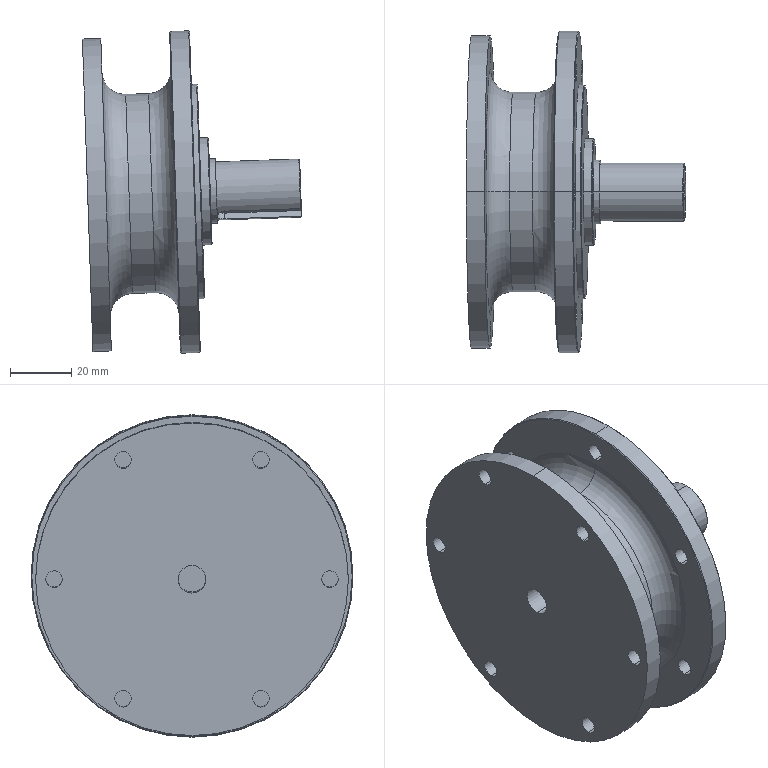Part | STEP file | 2026.6.15-Main Assembly图.sldasm-Part-92 | 1 solid | 73 faces | box 71.498 x 105 x 105.143 mm | volume 201131 mm3 | cylinder 45 | plane 13 | cone 11 | torus 4 | commonest cylinder face diameters 5.5 x24 5 x4 19 x3 9 x2 21 x2 35 x2